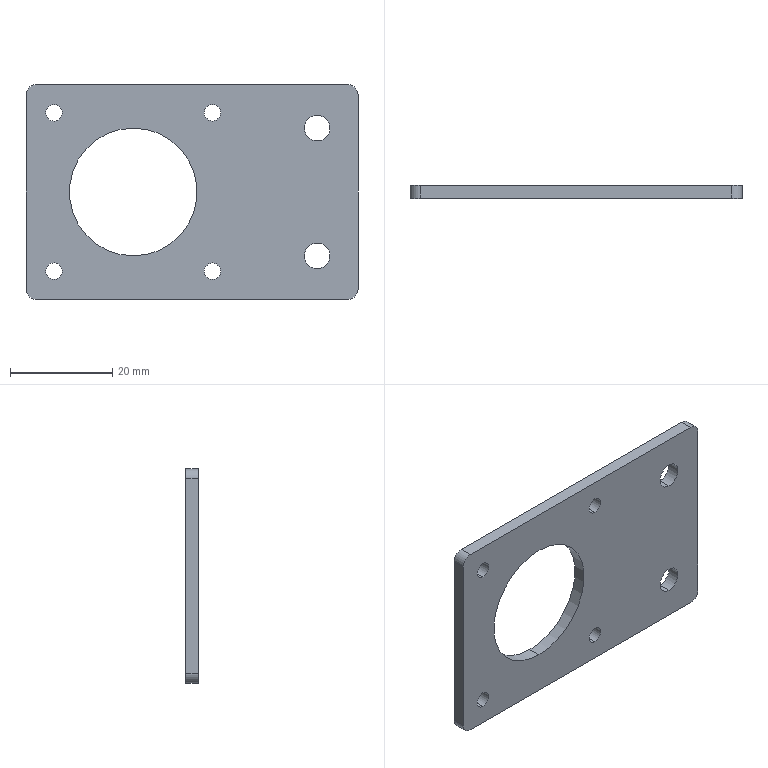Part | STEP file | 42 stepper aluminium flat bracket | 1 solid | 24 faces | box 65 x 2.5 x 42 mm | volume 5411 mm3 | cylinder 18 | plane 6 | commonest cylinder face diameters 3.2 x8 4 x4 5 x4 25 x2